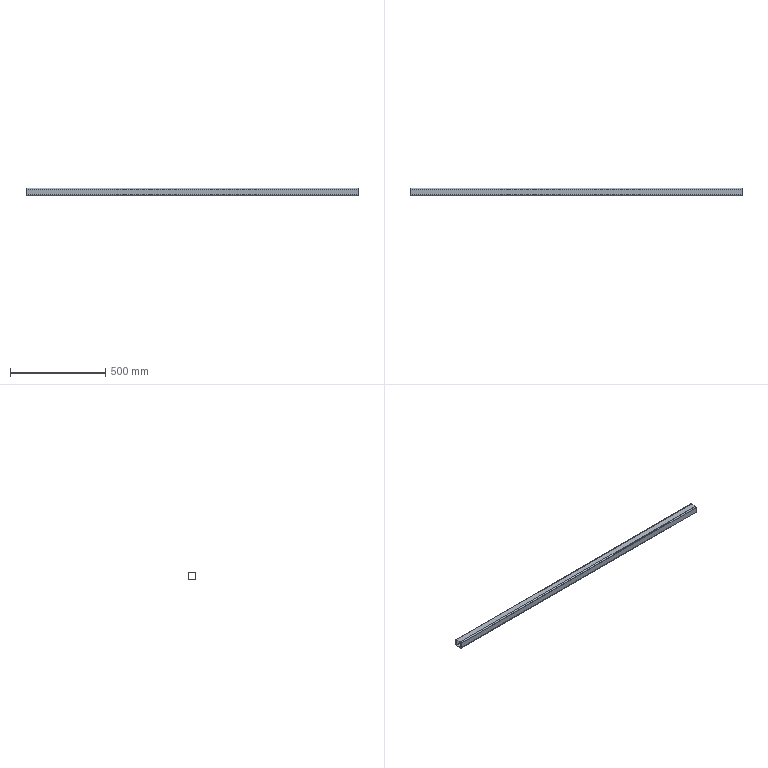Part | STEP file | SN10_002_008-04_TUBO_QUADRADO | 1 solid | 18 faces | box 1740 x 40 x 40 mm | volume 732232 mm3 | plane 10 | cylinder 8 | commonest cylinder face diameters 6 x4 12 x4
STEP:
#1=CARTESIAN_POINT('',(0.,0.,0.));
#2=DIRECTION('',(0.,0.,1.));
#3=DIRECTION('',(1.,0.,0.));
#4=AXIS2_PLACEMENT_3D('',#1,#2,#3);
#5=CARTESIAN_POINT('',(-870.,20.,14.));
#6=VERTEX_POINT('',#5);
#7=CARTESIAN_POINT('',(870.,20.,14.));
#8=VERTEX_POINT('',#7);
#9=CARTESIAN_POINT('',(-870.,20.,14.));
#10=DIRECTION('',(1.,0.,0.));
#11=VECTOR('',#10,1.);
#12=LINE('',#9,#11);
#13=CARTESIAN_POINT('',(0.,14.,14.));
#14=DIRECTION('',(1.,0.,0.));
#15=DIRECTION('',(0.,1.,0.));
#16=AXIS2_PLACEMENT_3D('',#13,#14,#15);
#17=CYLINDRICAL_SURFACE('',#16,6.);
#18=CARTESIAN_POINT('',(0.,-870.));
#19=DIRECTION('',(0.,1.));
#20=VECTOR('',#19,1.);
#21=LINE('',#18,#20);
#22=(GEOMETRIC_REPRESENTATION_CONTEXT(2)PARAMETRIC_REPRESENTATION_CONTEXT()REPRESENTATION_CONTEXT('',''));
#23=DEFINITIONAL_REPRESENTATION('',(#21),#22);
#24=PCURVE('',#17,#23);
#25=CARTESIAN_POINT('',(0.,20.,14.));
#26=DIRECTION('',(0.,-1.,0.));
#27=DIRECTION('',(0.,0.,-1.));
#28=AXIS2_PLACEMENT_3D('',#25,#26,#27);
#29=PLANE('',#28);
#30=CARTESIAN_POINT('',(0.,-870.));
#31=DIRECTION('',(0.,1.));
#32=VECTOR('',#31,1.);
#33=LINE('',#30,#32);
#34=(GEOMETRIC_REPRESENTATION_CONTEXT(2)PARAMETRIC_REPRESENTATION_CONTEXT()REPRESENTATION_CONTEXT('',''));
#35=DEFINITIONAL_REPRESENTATION('',(#33),#34);
#36=PCURVE('',#29,#35);
#37=SURFACE_CURVE('',#12,(#24,#36),.PCURVE_S1.);
#38=EDGE_CURVE('',#6,#8,#37,.T.);
#39=ORIENTED_EDGE('',*,*,#38,.F.);
#40=CARTESIAN_POINT('',(-870.,14.,20.));
#41=VERTEX_POINT('',#40);
#42=CARTESIAN_POINT('',(-870.,14.,14.));
#43=DIRECTION('',(1.,0.,0.));
#44=DIRECTION('',(0.,1.,0.));
#45=AXIS2_PLACEMENT_3D('',#42,#43,#44);
#46=CIRCLE('',#45,6.);
#47=CARTESIAN_POINT('',(0.,-870.));
#48=DIRECTION('',(1.,0.));
#49=VECTOR('',#48,1.);
#50=LINE('',#47,#49);
#51=(GEOMETRIC_REPRESENTATION_CONTEXT(2)PARAMETRIC_REPRESENTATION_CONTEXT()REPRESENTATION_CONTEXT('',''));
#52=DEFINITIONAL_REPRESENTATION('',(#50),#51);
#53=PCURVE('',#17,#52);
#54=CARTESIAN_POINT('',(-870.,0.,0.));
#55=DIRECTION('',(1.,0.,0.));
#56=DIRECTION('',(0.,0.,-1.));
#57=AXIS2_PLACEMENT_3D('',#54,#55,#56);
#58=PLANE('',#57);
#59=CARTESIAN_POINT('',(-14.,14.));
#60=DIRECTION('',(0.,1.));
#61=AXIS2_PLACEMENT_2D('',#59,#60);
#62=CIRCLE('',#61,6.);
#63=(GEOMETRIC_REPRESENTATION_CONTEXT(2)PARAMETRIC_REPRESENTATION_CONTEXT()REPRESENTATION_CONTEXT('',''));
#64=DEFINITIONAL_REPRESENTATION('',(#62),#63);
#65=PCURVE('',#58,#64);
#66=SURFACE_CURVE('',#46,(#53,#65),.PCURVE_S1.);
#67=EDGE_CURVE('',#6,#41,#66,.T.);
#68=ORIENTED_EDGE('',*,*,#67,.T.);
#69=CARTESIAN_POINT('',(870.,14.,20.));
#70=VERTEX_POINT('',#69);
#71=CARTESIAN_POINT('',(-870.,14.,20.));
#72=DIRECTION('',(1.,0.,0.));
#73=VECTOR('',#72,1.);
#74=LINE('',#71,#73);
#75=CARTESIAN_POINT('',(1.571,-870.));
#76=DIRECTION('',(0.,1.));
#77=VECTOR('',#76,1.);
#78=LINE('',#75,#77);
#79=(GEOMETRIC_REPRESENTATION_CONTEXT(2)PARAMETRIC_REPRESENTATION_CONTEXT()REPRESENTATION_CONTEXT('',''));
#80=DEFINITIONAL_REPRESENTATION('',(#78),#79);
#81=PCURVE('',#17,#80);
#82=CARTESIAN_POINT('',(0.,-14.,20.));
#83=DIRECTION('',(0.,0.,-1.));
#84=DIRECTION('',(-1.,0.,0.));
#85=AXIS2_PLACEMENT_3D('',#82,#83,#84);
#86=PLANE('',#85);
#87=CARTESIAN_POINT('',(870.,28.));
#88=DIRECTION('',(-1.,0.));
#89=VECTOR('',#88,1.);
#90=LINE('',#87,#89);
#91=(GEOMETRIC_REPRESENTATION_CONTEXT(2)PARAMETRIC_REPRESENTATION_CONTEXT()REPRESENTATION_CONTEXT('',''));
#92=DEFINITIONAL_REPRESENTATION('',(#90),#91);
#93=PCURVE('',#86,#92);
#94=SURFACE_CURVE('',#74,(#81,#93),.PCURVE_S1.);
#95=EDGE_CURVE('',#41,#70,#94,.T.);
#96=ORIENTED_EDGE('',*,*,#95,.T.);
#97=CARTESIAN_POINT('',(870.,14.,14.));
#98=DIRECTION('',(1.,0.,0.));
#99=DIRECTION('',(0.,1.,0.));
#100=AXIS2_PLACEMENT_3D('',#97,#98,#99);
#101=CIRCLE('',#100,6.);
#102=CARTESIAN_POINT('',(0.,870.));
#103=DIRECTION('',(1.,0.));
#104=VECTOR('',#103,1.);
#105=LINE('',#102,#104);
#106=(GEOMETRIC_REPRESENTATION_CONTEXT(2)PARAMETRIC_REPRESENTATION_CONTEXT()REPRESENTATION_CONTEXT('',''));
#107=DEFINITIONAL_REPRESENTATION('',(#105),#106);
#108=PCURVE('',#17,#107);
#109=CARTESIAN_POINT('',(870.,0.,0.));
#110=DIRECTION('',(1.,0.,0.));
#111=DIRECTION('',(0.,0.,-1.));
#112=AXIS2_PLACEMENT_3D('',#109,#110,#111);
#113=PLANE('',#112);
#114=CARTESIAN_POINT('',(-14.,14.));
#115=DIRECTION('',(0.,1.));
#116=AXIS2_PLACEMENT_2D('',#114,#115);
#117=CIRCLE('',#116,6.);
#118=(GEOMETRIC_REPRESENTATION_CONTEXT(2)PARAMETRIC_REPRESENTATION_CONTEXT()REPRESENTATION_CONTEXT('',''));
#119=DEFINITIONAL_REPRESENTATION('',(#117),#118);
#120=PCURVE('',#113,#119);
#121=SURFACE_CURVE('',#101,(#108,#120),.PCURVE_S1.);
#122=EDGE_CURVE('',#8,#70,#121,.T.);
#123=ORIENTED_EDGE('',*,*,#122,.F.);
#124=EDGE_LOOP('',(#39,#68,#96,#123));
#125=FACE_BOUND('',#124,.T.);
#126=ADVANCED_FACE('',(#125),#17,.T.);
#127=ORIENTED_EDGE('',*,*,#95,.F.);
#128=CARTESIAN_POINT('',(-870.,-14.,20.));
#129=VERTEX_POINT('',#128);
#130=CARTESIAN_POINT('',(-870.,-14.,20.));
#131=DIRECTION('',(0.,1.,0.));
#132=VECTOR('',#131,1.);
#133=LINE('',#130,#132);
#134=CARTESIAN_POINT('',(870.,0.));
#135=DIRECTION('',(0.,1.));
#136=VECTOR('',#135,1.);
#137=LINE('',#134,#136);
#138=(GEOMETRIC_REPRESENTATION_CONTEXT(2)PARAMETRIC_REPRESENTATION_CONTEXT()REPRESENTATION_CONTEXT('',''));
#139=DEFINITIONAL_REPRESENTATION('',(#137),#138);
#140=PCURVE('',#86,#139);
#141=CARTESIAN_POINT('',(-20.,-14.));
#142=DIRECTION('',(0.,1.));
#143=VECTOR('',#142,1.);
#144=LINE('',#141,#143);
#145=(GEOMETRIC_REPRESENTATION_CONTEXT(2)PARAMETRIC_REPRESENTATION_CONTEXT()REPRESENTATION_CONTEXT('',''));
#146=DEFINITIONAL_REPRESENTATION('',(#144),#145);
#147=PCURVE('',#58,#146);
#148=SURFACE_CURVE('',#133,(#140,#147),.PCURVE_S1.);
#149=EDGE_CURVE('',#129,#41,#148,.T.);
#150=ORIENTED_EDGE('',*,*,#149,.F.);
#151=CARTESIAN_POINT('',(870.,-14.,20.));
#152=VERTEX_POINT('',#151);
#153=CARTESIAN_POINT('',(-870.,-14.,20.));
#154=DIRECTION('',(1.,0.,0.));
#155=VECTOR('',#154,1.);
#156=LINE('',#153,#155);
#157=CARTESIAN_POINT('',(870.,0.));
#158=DIRECTION('',(-1.,0.));
#159=VECTOR('',#158,1.);
#160=LINE('',#157,#159);
#161=(GEOMETRIC_REPRESENTATION_CONTEXT(2)PARAMETRIC_REPRESENTATION_CONTEXT()REPRESENTATION_CONTEXT('',''));
#162=DEFINITIONAL_REPRESENTATION('',(#160),#161);
#163=PCURVE('',#86,#162);
#164=CARTESIAN_POINT('',(0.,-14.,14.));
#165=DIRECTION('',(1.,0.,0.));
#166=DIRECTION('',(0.,0.,1.));
#167=AXIS2_PLACEMENT_3D('',#164,#165,#166);
#168=CYLINDRICAL_SURFACE('',#167,6.);
#169=CARTESIAN_POINT('',(0.,-870.));
#170=DIRECTION('',(0.,1.));
#171=VECTOR('',#170,1.);
#172=LINE('',#169,#171);
#173=(GEOMETRIC_REPRESENTATION_CONTEXT(2)PARAMETRIC_REPRESENTATION_CONTEXT()REPRESENTATION_CONTEXT('',''));
#174=DEFINITIONAL_REPRESENTATION('',(#172),#173);
#175=PCURVE('',#168,#174);
#176=SURFACE_CURVE('',#156,(#163,#175),.PCURVE_S1.);
#177=EDGE_CURVE('',#129,#152,#176,.T.);
#178=ORIENTED_EDGE('',*,*,#177,.T.);
#179=CARTESIAN_POINT('',(870.,-14.,20.));
#180=DIRECTION('',(0.,1.,0.));
#181=VECTOR('',#180,1.);
#182=LINE('',#179,#181);
#183=CARTESIAN_POINT('',(-870.,0.));
#184=DIRECTION('',(0.,1.));
#185=VECTOR('',#184,1.);
#186=LINE('',#183,#185);
#187=(GEOMETRIC_REPRESENTATION_CONTEXT(2)PARAMETRIC_REPRESENTATION_CONTEXT()REPRESENTATION_CONTEXT('',''));
#188=DEFINITIONAL_REPRESENTATION('',(#186),#187);
#189=PCURVE('',#86,#188);
#190=CARTESIAN_POINT('',(-20.,-14.));
#191=DIRECTION('',(0.,1.));
#192=VECTOR('',#191,1.);
#193=LINE('',#190,#192);
#194=(GEOMETRIC_REPRESENTATION_CONTEXT(2)PARAMETRIC_REPRESENTATION_CONTEXT()REPRESENTATION_CONTEXT('',''));
#195=DEFINITIONAL_REPRESENTATION('',(#193),#194);
#196=PCURVE('',#113,#195);
#197=SURFACE_CURVE('',#182,(#189,#196),.PCURVE_S1.);
#198=EDGE_CURVE('',#152,#70,#197,.T.);
#199=ORIENTED_EDGE('',*,*,#198,.T.);
#200=EDGE_LOOP('',(#127,#150,#178,#199));
#201=FACE_BOUND('',#200,.T.);
#202=ADVANCED_FACE('',(#201),#86,.F.);
#203=ORIENTED_EDGE('',*,*,#177,.F.);
#204=CARTESIAN_POINT('',(-870.,-20.,14.));
#205=VERTEX_POINT('',#204);
#206=CARTESIAN_POINT('',(-870.,-14.,14.));
#207=DIRECTION('',(1.,0.,0.));
#208=DIRECTION('',(0.,1.,0.));
#209=AXIS2_PLACEMENT_3D('',#206,#207,#208);
#210=CIRCLE('',#209,6.);
#211=CARTESIAN_POINT('',(-1.571,-870.));
#212=DIRECTION('',(1.,0.));
#213=VECTOR('',#212,1.);
#214=LINE('',#211,#213);
#215=(GEOMETRIC_REPRESENTATION_CONTEXT(2)PARAMETRIC_REPRESENTATION_CONTEXT()REPRESENTATION_CONTEXT('',''));
#216=DEFINITIONAL_REPRESENTATION('',(#214),#215);
#217=PCURVE('',#168,#216);
#218=CARTESIAN_POINT('',(-14.,-14.));
#219=DIRECTION('',(0.,1.));
#220=AXIS2_PLACEMENT_2D('',#218,#219);
#221=CIRCLE('',#220,6.);
#222=(GEOMETRIC_REPRESENTATION_CONTEXT(2)PARAMETRIC_REPRESENTATION_CONTEXT()REPRESENTATION_CONTEXT('',''));
#223=DEFINITIONAL_REPRESENTATION('',(#221),#222);
#224=PCURVE('',#58,#223);
#225=SURFACE_CURVE('',#210,(#217,#224),.PCURVE_S1.);
#226=EDGE_CURVE('',#129,#205,#225,.T.);
#227=ORIENTED_EDGE('',*,*,#226,.T.);
#228=CARTESIAN_POINT('',(870.,-20.,14.));
#229=VERTEX_POINT('',#228);
#230=CARTESIAN_POINT('',(-870.,-20.,14.));
#231=DIRECTION('',(1.,0.,0.));
#232=VECTOR('',#231,1.);
#233=LINE('',#230,#232);
#234=CARTESIAN_POINT('',(1.571,-870.));
#235=DIRECTION('',(0.,1.));
#236=VECTOR('',#235,1.);
#237=LINE('',#234,#236);
#238=(GEOMETRIC_REPRESENTATION_CONTEXT(2)PARAMETRIC_REPRESENTATION_CONTEXT()REPRESENTATION_CONTEXT('',''));
#239=DEFINITIONAL_REPRESENTATION('',(#237),#238);
#240=PCURVE('',#168,#239);
#241=CARTESIAN_POINT('',(0.,-20.,-14.));
#242=DIRECTION('',(0.,1.,0.));
#243=DIRECTION('',(0.,0.,1.));
#244=AXIS2_PLACEMENT_3D('',#241,#242,#243);
#245=PLANE('',#244);
#246=CARTESIAN_POINT('',(28.,-870.));
#247=DIRECTION('',(0.,1.));
#248=VECTOR('',#247,1.);
#249=LINE('',#246,#248);
#250=(GEOMETRIC_REPRESENTATION_CONTEXT(2)PARAMETRIC_REPRESENTATION_CONTEXT()REPRESENTATION_CONTEXT('',''));
#251=DEFINITIONAL_REPRESENTATION('',(#249),#250);
#252=PCURVE('',#245,#251);
#253=SURFACE_CURVE('',#233,(#240,#252),.PCURVE_S1.);
#254=EDGE_CURVE('',#205,#229,#253,.T.);
#255=ORIENTED_EDGE('',*,*,#254,.T.);
#256=CARTESIAN_POINT('',(870.,-14.,14.));
#257=DIRECTION('',(1.,0.,0.));
#258=DIRECTION('',(0.,1.,0.));
#259=AXIS2_PLACEMENT_3D('',#256,#257,#258);
#260=CIRCLE('',#259,6.);
#261=CARTESIAN_POINT('',(-1.571,870.));
#262=DIRECTION('',(1.,0.));
#263=VECTOR('',#262,1.);
#264=LINE('',#261,#263);
#265=(GEOMETRIC_REPRESENTATION_CONTEXT(2)PARAMETRIC_REPRESENTATION_CONTEXT()REPRESENTATION_CONTEXT('',''));
#266=DEFINITIONAL_REPRESENTATION('',(#264),#265);
#267=PCURVE('',#168,#266);
#268=CARTESIAN_POINT('',(-14.,-14.));
#269=DIRECTION('',(0.,1.));
#270=AXIS2_PLACEMENT_2D('',#268,#269);
#271=CIRCLE('',#270,6.);
#272=(GEOMETRIC_REPRESENTATION_CONTEXT(2)PARAMETRIC_REPRESENTATION_CONTEXT()REPRESENTATION_CONTEXT('',''));
#273=DEFINITIONAL_REPRESENTATION('',(#271),#272);
#274=PCURVE('',#113,#273);
#275=SURFACE_CURVE('',#260,(#267,#274),.PCURVE_S1.);
#276=EDGE_CURVE('',#152,#229,#275,.T.);
#277=ORIENTED_EDGE('',*,*,#276,.F.);
#278=EDGE_LOOP('',(#203,#227,#255,#277));
#279=FACE_BOUND('',#278,.T.);
#280=ADVANCED_FACE('',(#279),#168,.T.);
#281=ORIENTED_EDGE('',*,*,#254,.F.);
#282=CARTESIAN_POINT('',(-870.,-20.,-14.));
#283=VERTEX_POINT('',#282);
#284=CARTESIAN_POINT('',(-870.,-20.,-14.));
#285=DIRECTION('',(0.,0.,1.));
#286=VECTOR('',#285,1.);
#287=LINE('',#284,#286);
#288=CARTESIAN_POINT('',(0.,-870.));
#289=DIRECTION('',(1.,0.));
#290=VECTOR('',#289,1.);
#291=LINE('',#288,#290);
#292=(GEOMETRIC_REPRESENTATION_CONTEXT(2)PARAMETRIC_REPRESENTATION_CONTEXT()REPRESENTATION_CONTEXT('',''));
#293=DEFINITIONAL_REPRESENTATION('',(#291),#292);
#294=PCURVE('',#245,#293);
#295=CARTESIAN_POINT('',(14.,-20.));
#296=DIRECTION('',(-1.,0.));
#297=VECTOR('',#296,1.);
#298=LINE('',#295,#297);
#299=(GEOMETRIC_REPRESENTATION_CONTEXT(2)PARAMETRIC_REPRESENTATION_CONTEXT()REPRESENTATION_CONTEXT('',''));
#300=DEFINITIONAL_REPRESENTATION('',(#298),#299);
#301=PCURVE('',#58,#300);
#302=SURFACE_CURVE('',#287,(#294,#301),.PCURVE_S1.);
#303=EDGE_CURVE('',#283,#205,#302,.T.);
#304=ORIENTED_EDGE('',*,*,#303,.F.);
#305=CARTESIAN_POINT('',(870.,-20.,-14.));
#306=VERTEX_POINT('',#305);
#307=CARTESIAN_POINT('',(-870.,-20.,-14.));
#308=DIRECTION('',(1.,0.,0.));
#309=VECTOR('',#308,1.);
#310=LINE('',#307,#309);
#311=CARTESIAN_POINT('',(0.,-870.));
#312=DIRECTION('',(0.,1.));
#313=VECTOR('',#312,1.);
#314=LINE('',#311,#313);
#315=(GEOMETRIC_REPRESENTATION_CONTEXT(2)PARAMETRIC_REPRESENTATION_CONTEXT()REPRESENTATION_CONTEXT('',''));
#316=DEFINITIONAL_REPRESENTATION('',(#314),#315);
#317=PCURVE('',#245,#316);
#318=CARTESIAN_POINT('',(0.,-14.,-14.));
#319=DIRECTION('',(1.,0.,0.));
#320=DIRECTION('',(0.,-1.,0.));
#321=AXIS2_PLACEMENT_3D('',#318,#319,#320);
#322=CYLINDRICAL_SURFACE('',#321,6.);
#323=CARTESIAN_POINT('',(0.,-870.));
#324=DIRECTION('',(0.,1.));
#325=VECTOR('',#324,1.);
#326=LINE('',#323,#325);
#327=(GEOMETRIC_REPRESENTATION_CONTEXT(2)PARAMETRIC_REPRESENTATION_CONTEXT()REPRESENTATION_CONTEXT('',''));
#328=DEFINITIONAL_REPRESENTATION('',(#326),#327);
#329=PCURVE('',#322,#328);
#330=SURFACE_CURVE('',#310,(#317,#329),.PCURVE_S1.);
#331=EDGE_CURVE('',#283,#306,#330,.T.);
#332=ORIENTED_EDGE('',*,*,#331,.T.);
#333=CARTESIAN_POINT('',(870.,-20.,-14.));
#334=DIRECTION('',(0.,0.,1.));
#335=VECTOR('',#334,1.);
#336=LINE('',#333,#335);
#337=CARTESIAN_POINT('',(0.,870.));
#338=DIRECTION('',(1.,0.));
#339=VECTOR('',#338,1.);
#340=LINE('',#337,#339);
#341=(GEOMETRIC_REPRESENTATION_CONTEXT(2)PARAMETRIC_REPRESENTATION_CONTEXT()REPRESENTATION_CONTEXT('',''));
#342=DEFINITIONAL_REPRESENTATION('',(#340),#341);
#343=PCURVE('',#245,#342);
#344=CARTESIAN_POINT('',(14.,-20.));
#345=DIRECTION('',(-1.,0.));
#346=VECTOR('',#345,1.);
#347=LINE('',#344,#346);
#348=(GEOMETRIC_REPRESENTATION_CONTEXT(2)PARAMETRIC_REPRESENTATION_CONTEXT()REPRESENTATION_CONTEXT('',''));
#349=DEFINITIONAL_REPRESENTATION('',(#347),#348);
#350=PCURVE('',#113,#349);
#351=SURFACE_CURVE('',#336,(#343,#350),.PCURVE_S1.);
#352=EDGE_CURVE('',#306,#229,#351,.T.);
#353=ORIENTED_EDGE('',*,*,#352,.T.);
#354=EDGE_LOOP('',(#281,#304,#332,#353));
#355=FACE_BOUND('',#354,.T.);
#356=ADVANCED_FACE('',(#355),#245,.F.);
#357=ORIENTED_EDGE('',*,*,#331,.F.);
#358=CARTESIAN_POINT('',(-870.,-14.,-20.));
#359=VERTEX_POINT('',#358);
#360=CARTESIAN_POINT('',(-870.,-14.,-14.));
#361=DIRECTION('',(1.,0.,0.));
#362=DIRECTION('',(0.,1.,0.));
#363=AXIS2_PLACEMENT_3D('',#360,#361,#362);
#364=CIRCLE('',#363,6.);
#365=CARTESIAN_POINT('',(-3.142,-870.));
#366=DIRECTION('',(1.,0.));
#367=VECTOR('',#366,1.);
#368=LINE('',#365,#367);
#369=(GEOMETRIC_REPRESENTATION_CONTEXT(2)PARAMETRIC_REPRESENTATION_CONTEXT()REPRESENTATION_CONTEXT('',''));
#370=DEFINITIONAL_REPRESENTATION('',(#368),#369);
#371=PCURVE('',#322,#370);
#372=CARTESIAN_POINT('',(14.,-14.));
#373=DIRECTION('',(0.,1.));
#374=AXIS2_PLACEMENT_2D('',#372,#373);
#375=CIRCLE('',#374,6.);
#376=(GEOMETRIC_REPRESENTATION_CONTEXT(2)PARAMETRIC_REPRESENTATION_CONTEXT()REPRESENTATION_CONTEXT('',''));
#377=DEFINITIONAL_REPRESENTATION('',(#375),#376);
#378=PCURVE('',#58,#377);
#379=SURFACE_CURVE('',#364,(#371,#378),.PCURVE_S1.);
#380=EDGE_CURVE('',#283,#359,#379,.T.);
#381=ORIENTED_EDGE('',*,*,#380,.T.);
#382=CARTESIAN_POINT('',(870.,-14.,-20.));
#383=VERTEX_POINT('',#382);
#384=CARTESIAN_POINT('',(-870.,-14.,-20.));
#385=DIRECTION('',(1.,0.,0.));
#386=VECTOR('',#385,1.);
#387=LINE('',#384,#386);
#388=CARTESIAN_POINT('',(1.571,-870.));
#389=DIRECTION('',(0.,1.));
#390=VECTOR('',#389,1.);
#391=LINE('',#388,#390);
#392=(GEOMETRIC_REPRESENTATION_CONTEXT(2)PARAMETRIC_REPRESENTATION_CONTEXT()REPRESENTATION_CONTEXT('',''));
#393=DEFINITIONAL_REPRESENTATION('',(#391),#392);
#394=PCURVE('',#322,#393);
#395=CARTESIAN_POINT('',(0.,14.,-20.));
#396=DIRECTION('',(0.,0.,1.));
#397=DIRECTION('',(1.,0.,0.));
#398=AXIS2_PLACEMENT_3D('',#395,#396,#397);
#399=PLANE('',#398);
#400=CARTESIAN_POINT('',(-870.,-28.));
#401=DIRECTION('',(1.,0.));
#402=VECTOR('',#401,1.);
#403=LINE('',#400,#402);
#404=(GEOMETRIC_REPRESENTATION_CONTEXT(2)PARAMETRIC_REPRESENTATION_CONTEXT()REPRESENTATION_CONTEXT('',''));
#405=DEFINITIONAL_REPRESENTATION('',(#403),#404);
#406=PCURVE('',#399,#405);
#407=SURFACE_CURVE('',#387,(#394,#406),.PCURVE_S1.);
#408=EDGE_CURVE('',#359,#383,#407,.T.);
#409=ORIENTED_EDGE('',*,*,#408,.T.);
#410=CARTESIAN_POINT('',(870.,-14.,-14.));
#411=DIRECTION('',(1.,0.,0.));
#412=DIRECTION('',(0.,1.,0.));
#413=AXIS2_PLACEMENT_3D('',#410,#411,#412);
#414=CIRCLE('',#413,6.);
#415=CARTESIAN_POINT('',(-3.142,870.));
#416=DIRECTION('',(1.,0.));
#417=VECTOR('',#416,1.);
#418=LINE('',#415,#417);
#419=(GEOMETRIC_REPRESENTATION_CONTEXT(2)PARAMETRIC_REPRESENTATION_CONTEXT()REPRESENTATION_CONTEXT('',''));
#420=DEFINITIONAL_REPRESENTATION('',(#418),#419);
#421=PCURVE('',#322,#420);
#422=CARTESIAN_POINT('',(14.,-14.));
#423=DIRECTION('',(0.,1.));
#424=AXIS2_PLACEMENT_2D('',#422,#423);
#425=CIRCLE('',#424,6.);
#426=(GEOMETRIC_REPRESENTATION_CONTEXT(2)PARAMETRIC_REPRESENTATION_CONTEXT()REPRESENTATION_CONTEXT('',''));
#427=DEFINITIONAL_REPRESENTATION('',(#425),#426);
#428=PCURVE('',#113,#427);
#429=SURFACE_CURVE('',#414,(#421,#428),.PCURVE_S1.);
#430=EDGE_CURVE('',#306,#383,#429,.T.);
#431=ORIENTED_EDGE('',*,*,#430,.F.);
#432=EDGE_LOOP('',(#357,#381,#409,#431));
#433=FACE_BOUND('',#432,.T.);
#434=ADVANCED_FACE('',(#433),#322,.T.);
#435=ORIENTED_EDGE('',*,*,#408,.F.);
#436=CARTESIAN_POINT('',(-870.,14.,-20.));
#437=VERTEX_POINT('',#436);
#438=CARTESIAN_POINT('',(-870.,14.,-20.));
#439=DIRECTION('',(0.,-1.,0.));
#440=VECTOR('',#439,1.);
#441=LINE('',#438,#440);
#442=CARTESIAN_POINT('',(-870.,0.));
#443=DIRECTION('',(0.,-1.));
#444=VECTOR('',#443,1.);
#445=LINE('',#442,#444);
#446=(GEOMETRIC_REPRESENTATION_CONTEXT(2)PARAMETRIC_REPRESENTATION_CONTEXT()REPRESENTATION_CONTEXT('',''));
#447=DEFINITIONAL_REPRESENTATION('',(#445),#446);
#448=PCURVE('',#399,#447);
#449=CARTESIAN_POINT('',(20.,14.));
#450=DIRECTION('',(0.,-1.));
#451=VECTOR('',#450,1.);
#452=LINE('',#449,#451);
#453=(GEOMETRIC_REPRESENTATION_CONTEXT(2)PARAMETRIC_REPRESENTATION_CONTEXT()REPRESENTATION_CONTEXT('',''));
#454=DEFINITIONAL_REPRESENTATION('',(#452),#453);
#455=PCURVE('',#58,#454);
#456=SURFACE_CURVE('',#441,(#448,#455),.PCURVE_S1.);
#457=EDGE_CURVE('',#437,#359,#456,.T.);
#458=ORIENTED_EDGE('',*,*,#457,.F.);
#459=CARTESIAN_POINT('',(870.,14.,-20.));
#460=VERTEX_POINT('',#459);
#461=CARTESIAN_POINT('',(-870.,14.,-20.));
#462=DIRECTION('',(1.,0.,0.));
#463=VECTOR('',#462,1.);
#464=LINE('',#461,#463);
#465=CARTESIAN_POINT('',(-870.,0.));
#466=DIRECTION('',(1.,0.));
#467=VECTOR('',#466,1.);
#468=LINE('',#465,#467);
#469=(GEOMETRIC_REPRESENTATION_CONTEXT(2)PARAMETRIC_REPRESENTATION_CONTEXT()REPRESENTATION_CONTEXT('',''));
#470=DEFINITIONAL_REPRESENTATION('',(#468),#469);
#471=PCURVE('',#399,#470);
#472=CARTESIAN_POINT('',(0.,14.,-14.));
#473=DIRECTION('',(1.,0.,0.));
#474=DIRECTION('',(0.,0.,-1.));
#475=AXIS2_PLACEMENT_3D('',#472,#473,#474);
#476=CYLINDRICAL_SURFACE('',#475,6.);
#477=CARTESIAN_POINT('',(0.,-870.));
#478=DIRECTION('',(0.,1.));
#479=VECTOR('',#478,1.);
#480=LINE('',#477,#479);
#481=(GEOMETRIC_REPRESENTATION_CONTEXT(2)PARAMETRIC_REPRESENTATION_CONTEXT()REPRESENTATION_CONTEXT('',''));
#482=DEFINITIONAL_REPRESENTATION('',(#480),#481);
#483=PCURVE('',#476,#482);
#484=SURFACE_CURVE('',#464,(#471,#483),.PCURVE_S1.);
#485=EDGE_CURVE('',#437,#460,#484,.T.);
#486=ORIENTED_EDGE('',*,*,#485,.T.);
#487=CARTESIAN_POINT('',(870.,14.,-20.));
#488=DIRECTION('',(0.,-1.,0.));
#489=VECTOR('',#488,1.);
#490=LINE('',#487,#489);
#491=CARTESIAN_POINT('',(870.,0.));
#492=DIRECTION('',(0.,-1.));
#493=VECTOR('',#492,1.);
#494=LINE('',#491,#493);
#495=(GEOMETRIC_REPRESENTATION_CONTEXT(2)PARAMETRIC_REPRESENTATION_CONTEXT()REPRESENTATION_CONTEXT('',''));
#496=DEFINITIONAL_REPRESENTATION('',(#494),#495);
#497=PCURVE('',#399,#496);
#498=CARTESIAN_POINT('',(20.,14.));
#499=DIRECTION('',(0.,-1.));
#500=VECTOR('',#499,1.);
#501=LINE('',#498,#500);
#502=(GEOMETRIC_REPRESENTATION_CONTEXT(2)PARAMETRIC_REPRESENTATION_CONTEXT()REPRESENTATION_CONTEXT('',''));
#503=DEFINITIONAL_REPRESENTATION('',(#501),#502);
#504=PCURVE('',#113,#503);
#505=SURFACE_CURVE('',#490,(#497,#504),.PCURVE_S1.);
#506=EDGE_CURVE('',#460,#383,#505,.T.);
#507=ORIENTED_EDGE('',*,*,#506,.T.);
#508=EDGE_LOOP('',(#435,#458,#486,#507));
#509=FACE_BOUND('',#508,.T.);
#510=ADVANCED_FACE('',(#509),#399,.F.);
#511=ORIENTED_EDGE('',*,*,#485,.F.);
#512=CARTESIAN_POINT('',(-870.,20.,-14.));
#513=VERTEX_POINT('',#512);
#514=CARTESIAN_POINT('',(-870.,14.,-14.));
#515=DIRECTION('',(1.,0.,0.));
#516=DIRECTION('',(0.,1.,0.));
#517=AXIS2_PLACEMENT_3D('',#514,#515,#516);
#518=CIRCLE('',#517,6.);
#519=CARTESIAN_POINT('',(-4.712,-870.));
#520=DIRECTION('',(1.,0.));
#521=VECTOR('',#520,1.);
#522=LINE('',#519,#521);
#523=(GEOMETRIC_REPRESENTATION_CONTEXT(2)PARAMETRIC_REPRESENTATION_CONTEXT()REPRESENTATION_CONTEXT('',''));
#524=DEFINITIONAL_REPRESENTATION('',(#522),#523);
#525=PCURVE('',#476,#524);
#526=CARTESIAN_POINT('',(14.,14.));
#527=DIRECTION('',(0.,1.));
#528=AXIS2_PLACEMENT_2D('',#526,#527);
#529=CIRCLE('',#528,6.);
#530=(GEOMETRIC_REPRESENTATION_CONTEXT(2)PARAMETRIC_REPRESENTATION_CONTEXT()REPRESENTATION_CONTEXT('',''));
#531=DEFINITIONAL_REPRESENTATION('',(#529),#530);
#532=PCURVE('',#58,#531);
#533=SURFACE_CURVE('',#518,(#525,#532),.PCURVE_S1.);
#534=EDGE_CURVE('',#437,#513,#533,.T.);
#535=ORIENTED_EDGE('',*,*,#534,.T.);
#536=CARTESIAN_POINT('',(870.,20.,-14.));
#537=VERTEX_POINT('',#536);
#538=CARTESIAN_POINT('',(-870.,20.,-14.));
#539=DIRECTION('',(1.,0.,0.));
#540=VECTOR('',#539,1.);
#541=LINE('',#538,#540);
#542=CARTESIAN_POINT('',(1.571,-870.));
#543=DIRECTION('',(0.,1.));
#544=VECTOR('',#543,1.);
#545=LINE('',#542,#544);
#546=(GEOMETRIC_REPRESENTATION_CONTEXT(2)PARAMETRIC_REPRESENTATION_CONTEXT()REPRESENTATION_CONTEXT('',''));
#547=DEFINITIONAL_REPRESENTATION('',(#545),#546);
#548=PCURVE('',#476,#547);
#549=CARTESIAN_POINT('',(28.,-870.));
#550=DIRECTION('',(0.,1.));
#551=VECTOR('',#550,1.);
#552=LINE('',#549,#551);
#553=(GEOMETRIC_REPRESENTATION_CONTEXT(2)PARAMETRIC_REPRESENTATION_CONTEXT()REPRESENTATION_CONTEXT('',''));
#554=DEFINITIONAL_REPRESENTATION('',(#552),#553);
#555=PCURVE('',#29,#554);
#556=SURFACE_CURVE('',#541,(#548,#555),.PCURVE_S1.);
#557=EDGE_CURVE('',#513,#537,#556,.T.);
#558=ORIENTED_EDGE('',*,*,#557,.T.);
#559=CARTESIAN_POINT('',(870.,14.,-14.));
#560=DIRECTION('',(1.,0.,0.));
#561=DIRECTION('',(0.,1.,0.));
#562=AXIS2_PLACEMENT_3D('',#559,#560,#561);
#563=CIRCLE('',#562,6.);
#564=CARTESIAN_POINT('',(-4.712,870.));
#565=DIRECTION('',(1.,0.));
#566=VECTOR('',#565,1.);
#567=LINE('',#564,#566);
#568=(GEOMETRIC_REPRESENTATION_CONTEXT(2)PARAMETRIC_REPRESENTATION_CONTEXT()REPRESENTATION_CONTEXT('',''));
#569=DEFINITIONAL_REPRESENTATION('',(#567),#568);
#570=PCURVE('',#476,#569);
#571=CARTESIAN_POINT('',(14.,14.));
#572=DIRECTION('',(0.,1.));
#573=AXIS2_PLACEMENT_2D('',#571,#572);
#574=CIRCLE('',#573,6.);
#575=(GEOMETRIC_REPRESENTATION_CONTEXT(2)PARAMETRIC_REPRESENTATION_CONTEXT()REPRESENTATION_CONTEXT('',''));
#576=DEFINITIONAL_REPRESENTATION('',(#574),#575);
#577=PCURVE('',#113,#576);
#578=SURFACE_CURVE('',#563,(#570,#577),.PCURVE_S1.);
#579=EDGE_CURVE('',#460,#537,#578,.T.);
#580=ORIENTED_EDGE('',*,*,#579,.F.);
#581=EDGE_LOOP('',(#511,#535,#558,#580));
#582=FACE_BOUND('',#581,.T.);
#583=ADVANCED_FACE('',(#582),#476,.T.);
#584=ORIENTED_EDGE('',*,*,#557,.F.);
#585=CARTESIAN_POINT('',(-870.,20.,14.));
#586=DIRECTION('',(0.,0.,-1.));
#587=VECTOR('',#586,1.);
#588=LINE('',#585,#587);
#589=CARTESIAN_POINT('',(0.,-870.));
#590=DIRECTION('',(1.,0.));
#591=VECTOR('',#590,1.);
#592=LINE('',#589,#591);
#593=(GEOMETRIC_REPRESENTATION_CONTEXT(2)PARAMETRIC_REPRESENTATION_CONTEXT()REPRESENTATION_CONTEXT('',''));
#594=DEFINITIONAL_REPRESENTATION('',(#592),#593);
#595=PCURVE('',#29,#594);
#596=CARTESIAN_POINT('',(-14.,20.));
#597=DIRECTION('',(1.,0.));
#598=VECTOR('',#597,1.);
#599=LINE('',#596,#598);
#600=(GEOMETRIC_REPRESENTATION_CONTEXT(2)PARAMETRIC_REPRESENTATION_CONTEXT()REPRESENTATION_CONTEXT('',''));
#601=DEFINITIONAL_REPRESENTATION('',(#599),#600);
#602=PCURVE('',#58,#601);
#603=SURFACE_CURVE('',#588,(#595,#602),.PCURVE_S1.);
#604=EDGE_CURVE('',#6,#513,#603,.T.);
#605=ORIENTED_EDGE('',*,*,#604,.F.);
#606=ORIENTED_EDGE('',*,*,#38,.T.);
#607=CARTESIAN_POINT('',(870.,20.,14.));
#608=DIRECTION('',(0.,0.,-1.));
#609=VECTOR('',#608,1.);
#610=LINE('',#607,#609);
#611=CARTESIAN_POINT('',(0.,870.));
#612=DIRECTION('',(1.,0.));
#613=VECTOR('',#612,1.);
#614=LINE('',#611,#613);
#615=(GEOMETRIC_REPRESENTATION_CONTEXT(2)PARAMETRIC_REPRESENTATION_CONTEXT()REPRESENTATION_CONTEXT('',''));
#616=DEFINITIONAL_REPRESENTATION('',(#614),#615);
#617=PCURVE('',#29,#616);
#618=CARTESIAN_POINT('',(-14.,20.));
#619=DIRECTION('',(1.,0.));
#620=VECTOR('',#619,1.);
#621=LINE('',#618,#620);
#622=(GEOMETRIC_REPRESENTATION_CONTEXT(2)PARAMETRIC_REPRESENTATION_CONTEXT()REPRESENTATION_CONTEXT('',''));
#623=DEFINITIONAL_REPRESENTATION('',(#621),#622);
#624=PCURVE('',#113,#623);
#625=SURFACE_CURVE('',#610,(#617,#624),.PCURVE_S1.);
#626=EDGE_CURVE('',#8,#537,#625,.T.);
#627=ORIENTED_EDGE('',*,*,#626,.T.);
#628=EDGE_LOOP('',(#584,#605,#606,#627));
#629=FACE_BOUND('',#628,.T.);
#630=ADVANCED_FACE('',(#629),#29,.F.);
#631=CARTESIAN_POINT('',(870.,17.,14.));
#632=VERTEX_POINT('',#631);
#633=CARTESIAN_POINT('',(870.,17.,-14.));
#634=VERTEX_POINT('',#633);
#635=CARTESIAN_POINT('',(870.,17.,14.));
#636=DIRECTION('',(0.,0.,-1.));
#637=VECTOR('',#636,1.);
#638=LINE('',#635,#637);
#639=CARTESIAN_POINT('',(0.,17.,14.));
#640=DIRECTION('',(0.,-1.,0.));
#641=DIRECTION('',(0.,0.,-1.));
#642=AXIS2_PLACEMENT_3D('',#639,#640,#641);
#643=PLANE('',#642);
#644=CARTESIAN_POINT('',(0.,870.));
#645=DIRECTION('',(1.,0.));
#646=VECTOR('',#645,1.);
#647=LINE('',#644,#646);
#648=(GEOMETRIC_REPRESENTATION_CONTEXT(2)PARAMETRIC_REPRESENTATION_CONTEXT()REPRESENTATION_CONTEXT('',''));
#649=DEFINITIONAL_REPRESENTATION('',(#647),#648);
#650=PCURVE('',#643,#649);
#651=CARTESIAN_POINT('',(-14.,17.));
#652=DIRECTION('',(1.,0.));
#653=VECTOR('',#652,1.);
#654=LINE('',#651,#653);
#655=(GEOMETRIC_REPRESENTATION_CONTEXT(2)PARAMETRIC_REPRESENTATION_CONTEXT()REPRESENTATION_CONTEXT('',''));
#656=DEFINITIONAL_REPRESENTATION('',(#654),#655);
#657=PCURVE('',#113,#656);
#658=SURFACE_CURVE('',#638,(#650,#657),.PCURVE_S1.);
#659=EDGE_CURVE('',#632,#634,#658,.T.);
#660=ORIENTED_EDGE('',*,*,#659,.F.);
#661=CARTESIAN_POINT('',(-870.,17.,14.));
#662=VERTEX_POINT('',#661);
#663=CARTESIAN_POINT('',(-870.,17.,14.));
#664=DIRECTION('',(1.,0.,0.));
#665=VECTOR('',#664,1.);
#666=LINE('',#663,#665);
#667=CARTESIAN_POINT('',(0.,-870.));
#668=DIRECTION('',(0.,1.));
#669=VECTOR('',#668,1.);
#670=LINE('',#667,#669);
#671=(GEOMETRIC_REPRESENTATION_CONTEXT(2)PARAMETRIC_REPRESENTATION_CONTEXT()REPRESENTATION_CONTEXT('',''));
#672=DEFINITIONAL_REPRESENTATION('',(#670),#671);
#673=PCURVE('',#643,#672);
#674=CARTESIAN_POINT('',(0.,14.,14.));
#675=DIRECTION('',(1.,0.,0.));
#676=DIRECTION('',(0.,1.,0.));
#677=AXIS2_PLACEMENT_3D('',#674,#675,#676);
#678=CYLINDRICAL_SURFACE('',#677,3.);
#679=CARTESIAN_POINT('',(0.,-870.));
#680=DIRECTION('',(0.,1.));
#681=VECTOR('',#680,1.);
#682=LINE('',#679,#681);
#683=(GEOMETRIC_REPRESENTATION_CONTEXT(2)PARAMETRIC_REPRESENTATION_CONTEXT()REPRESENTATION_CONTEXT('',''));
#684=DEFINITIONAL_REPRESENTATION('',(#682),#683);
#685=PCURVE('',#678,#684);
#686=SURFACE_CURVE('',#666,(#673,#685),.PCURVE_S1.);
#687=EDGE_CURVE('',#662,#632,#686,.T.);
#688=ORIENTED_EDGE('',*,*,#687,.F.);
#689=CARTESIAN_POINT('',(-870.,17.,-14.));
#690=VERTEX_POINT('',#689);
#691=CARTESIAN_POINT('',(-870.,17.,14.));
#692=DIRECTION('',(0.,0.,-1.));
#693=VECTOR('',#692,1.);
#694=LINE('',#691,#693);
#695=CARTESIAN_POINT('',(0.,-870.));
#696=DIRECTION('',(1.,0.));
#697=VECTOR('',#696,1.);
#698=LINE('',#695,#697);
#699=(GEOMETRIC_REPRESENTATION_CONTEXT(2)PARAMETRIC_REPRESENTATION_CONTEXT()REPRESENTATION_CONTEXT('',''));
#700=DEFINITIONAL_REPRESENTATION('',(#698),#699);
#701=PCURVE('',#643,#700);
#702=CARTESIAN_POINT('',(-14.,17.));
#703=DIRECTION('',(1.,0.));
#704=VECTOR('',#703,1.);
#705=LINE('',#702,#704);
#706=(GEOMETRIC_REPRESENTATION_CONTEXT(2)PARAMETRIC_REPRESENTATION_CONTEXT()REPRESENTATION_CONTEXT('',''));
#707=DEFINITIONAL_REPRESENTATION('',(#705),#706);
#708=PCURVE('',#58,#707);
#709=SURFACE_CURVE('',#694,(#701,#708),.PCURVE_S1.);
#710=EDGE_CURVE('',#662,#690,#709,.T.);
#711=ORIENTED_EDGE('',*,*,#710,.T.);
#712=CARTESIAN_POINT('',(-870.,17.,-14.));
#713=DIRECTION('',(1.,0.,0.));
#714=VECTOR('',#713,1.);
#715=LINE('',#712,#714);
#716=CARTESIAN_POINT('',(28.,-870.));
#717=DIRECTION('',(0.,1.));
#718=VECTOR('',#717,1.);
#719=LINE('',#716,#718);
#720=(GEOMETRIC_REPRESENTATION_CONTEXT(2)PARAMETRIC_REPRESENTATION_CONTEXT()REPRESENTATION_CONTEXT('',''));
#721=DEFINITIONAL_REPRESENTATION('',(#719),#720);
#722=PCURVE('',#643,#721);
#723=CARTESIAN_POINT('',(0.,14.,-14.));
#724=DIRECTION('',(1.,0.,0.));
#725=DIRECTION('',(0.,0.,-1.));
#726=AXIS2_PLACEMENT_3D('',#723,#724,#725);
#727=CYLINDRICAL_SURFACE('',#726,3.);
#728=CARTESIAN_POINT('',(1.571,-870.));
#729=DIRECTION('',(0.,1.));
#730=VECTOR('',#729,1.);
#731=LINE('',#728,#730);
#732=(GEOMETRIC_REPRESENTATION_CONTEXT(2)PARAMETRIC_REPRESENTATION_CONTEXT()REPRESENTATION_CONTEXT('',''));
#733=DEFINITIONAL_REPRESENTATION('',(#731),#732);
#734=PCURVE('',#727,#733);
#735=SURFACE_CURVE('',#715,(#722,#734),.PCURVE_S1.);
#736=EDGE_CURVE('',#690,#634,#735,.T.);
#737=ORIENTED_EDGE('',*,*,#736,.T.);
#738=EDGE_LOOP('',(#660,#688,#711,#737));
#739=FACE_BOUND('',#738,.T.);
#740=ADVANCED_FACE('',(#739),#643,.T.);
#741=CARTESIAN_POINT('',(-870.,14.,-17.));
#742=VERTEX_POINT('',#741);
#743=CARTESIAN_POINT('',(870.,14.,-17.));
#744=VERTEX_POINT('',#743);
#745=CARTESIAN_POINT('',(-870.,14.,-17.));
#746=DIRECTION('',(1.,0.,0.));
#747=VECTOR('',#746,1.);
#748=LINE('',#745,#747);
#749=CARTESIAN_POINT('',(0.,-870.));
#750=DIRECTION('',(0.,1.));
#751=VECTOR('',#750,1.);
#752=LINE('',#749,#751);
#753=(GEOMETRIC_REPRESENTATION_CONTEXT(2)PARAMETRIC_REPRESENTATION_CONTEXT()REPRESENTATION_CONTEXT('',''));
#754=DEFINITIONAL_REPRESENTATION('',(#752),#753);
#755=PCURVE('',#727,#754);
#756=CARTESIAN_POINT('',(0.,14.,-17.));
#757=DIRECTION('',(0.,0.,1.));
#758=DIRECTION('',(1.,0.,0.));
#759=AXIS2_PLACEMENT_3D('',#756,#757,#758);
#760=PLANE('',#759);
#761=CARTESIAN_POINT('',(-870.,0.));
#762=DIRECTION('',(1.,0.));
#763=VECTOR('',#762,1.);
#764=LINE('',#761,#763);
#765=(GEOMETRIC_REPRESENTATION_CONTEXT(2)PARAMETRIC_REPRESENTATION_CONTEXT()REPRESENTATION_CONTEXT('',''));
#766=DEFINITIONAL_REPRESENTATION('',(#764),#765);
#767=PCURVE('',#760,#766);
#768=SURFACE_CURVE('',#748,(#755,#767),.PCURVE_S1.);
#769=EDGE_CURVE('',#742,#744,#768,.T.);
#770=ORIENTED_EDGE('',*,*,#769,.F.);
#771=CARTESIAN_POINT('',(-870.,14.,-14.));
#772=DIRECTION('',(1.,0.,0.));
#773=DIRECTION('',(0.,1.,0.));
#774=AXIS2_PLACEMENT_3D('',#771,#772,#773);
#775=CIRCLE('',#774,3.);
#776=CARTESIAN_POINT('',(-4.712,-870.));
#777=DIRECTION('',(1.,0.));
#778=VECTOR('',#777,1.);
#779=LINE('',#776,#778);
#780=(GEOMETRIC_REPRESENTATION_CONTEXT(2)PARAMETRIC_REPRESENTATION_CONTEXT()REPRESENTATION_CONTEXT('',''));
#781=DEFINITIONAL_REPRESENTATION('',(#779),#780);
#782=PCURVE('',#727,#781);
#783=CARTESIAN_POINT('',(14.,14.));
#784=DIRECTION('',(0.,1.));
#785=AXIS2_PLACEMENT_2D('',#783,#784);
#786=CIRCLE('',#785,3.);
#787=(GEOMETRIC_REPRESENTATION_CONTEXT(2)PARAMETRIC_REPRESENTATION_CONTEXT()REPRESENTATION_CONTEXT('',''));
#788=DEFINITIONAL_REPRESENTATION('',(#786),#787);
#789=PCURVE('',#58,#788);
#790=SURFACE_CURVE('',#775,(#782,#789),.PCURVE_S1.);
#791=EDGE_CURVE('',#742,#690,#790,.T.);
#792=ORIENTED_EDGE('',*,*,#791,.T.);
#793=ORIENTED_EDGE('',*,*,#736,.T.);
#794=CARTESIAN_POINT('',(870.,14.,-14.));
#795=DIRECTION('',(1.,0.,0.));
#796=DIRECTION('',(0.,1.,0.));
#797=AXIS2_PLACEMENT_3D('',#794,#795,#796);
#798=CIRCLE('',#797,3.);
#799=CARTESIAN_POINT('',(-4.712,870.));
#800=DIRECTION('',(1.,0.));
#801=VECTOR('',#800,1.);
#802=LINE('',#799,#801);
#803=(GEOMETRIC_REPRESENTATION_CONTEXT(2)PARAMETRIC_REPRESENTATION_CONTEXT()REPRESENTATION_CONTEXT('',''));
#804=DEFINITIONAL_REPRESENTATION('',(#802),#803);
#805=PCURVE('',#727,#804);
#806=CARTESIAN_POINT('',(14.,14.));
#807=DIRECTION('',(0.,1.));
#808=AXIS2_PLACEMENT_2D('',#806,#807);
#809=CIRCLE('',#808,3.);
#810=(GEOMETRIC_REPRESENTATION_CONTEXT(2)PARAMETRIC_REPRESENTATION_CONTEXT()REPRESENTATION_CONTEXT('',''));
#811=DEFINITIONAL_REPRESENTATION('',(#809),#810);
#812=PCURVE('',#113,#811);
#813=SURFACE_CURVE('',#798,(#805,#812),.PCURVE_S1.);
#814=EDGE_CURVE('',#744,#634,#813,.T.);
#815=ORIENTED_EDGE('',*,*,#814,.F.);
#816=EDGE_LOOP('',(#770,#792,#793,#815));
#817=FACE_BOUND('',#816,.F.);
#818=ADVANCED_FACE('',(#817),#727,.F.);
#819=CARTESIAN_POINT('',(870.,-14.,-17.));
#820=VERTEX_POINT('',#819);
#821=CARTESIAN_POINT('',(870.,14.,-17.));
#822=DIRECTION('',(0.,-1.,0.));
#823=VECTOR('',#822,1.);
#824=LINE('',#821,#823);
#825=CARTESIAN_POINT('',(870.,0.));
#826=DIRECTION('',(0.,-1.));
#827=VECTOR('',#826,1.);
#828=LINE('',#825,#827);
#829=(GEOMETRIC_REPRESENTATION_CONTEXT(2)PARAMETRIC_REPRESENTATION_CONTEXT()REPRESENTATION_CONTEXT('',''));
#830=DEFINITIONAL_REPRESENTATION('',(#828),#829);
#831=PCURVE('',#760,#830);
#832=CARTESIAN_POINT('',(17.,14.));
#833=DIRECTION('',(0.,-1.));
#834=VECTOR('',#833,1.);
#835=LINE('',#832,#834);
#836=(GEOMETRIC_REPRESENTATION_CONTEXT(2)PARAMETRIC_REPRESENTATION_CONTEXT()REPRESENTATION_CONTEXT('',''));
#837=DEFINITIONAL_REPRESENTATION('',(#835),#836);
#838=PCURVE('',#113,#837);
#839=SURFACE_CURVE('',#824,(#831,#838),.PCURVE_S1.);
#840=EDGE_CURVE('',#744,#820,#839,.T.);
#841=ORIENTED_EDGE('',*,*,#840,.F.);
#842=ORIENTED_EDGE('',*,*,#769,.F.);
#843=CARTESIAN_POINT('',(-870.,-14.,-17.));
#844=VERTEX_POINT('',#843);
#845=CARTESIAN_POINT('',(-870.,14.,-17.));
#846=DIRECTION('',(0.,-1.,0.));
#847=VECTOR('',#846,1.);
#848=LINE('',#845,#847);
#849=CARTESIAN_POINT('',(-870.,0.));
#850=DIRECTION('',(0.,-1.));
#851=VECTOR('',#850,1.);
#852=LINE('',#849,#851);
#853=(GEOMETRIC_REPRESENTATION_CONTEXT(2)PARAMETRIC_REPRESENTATION_CONTEXT()REPRESENTATION_CONTEXT('',''));
#854=DEFINITIONAL_REPRESENTATION('',(#852),#853);
#855=PCURVE('',#760,#854);
#856=CARTESIAN_POINT('',(17.,14.));
#857=DIRECTION('',(0.,-1.));
#858=VECTOR('',#857,1.);
#859=LINE('',#856,#858);
#860=(GEOMETRIC_REPRESENTATION_CONTEXT(2)PARAMETRIC_REPRESENTATION_CONTEXT()REPRESENTATION_CONTEXT('',''));
#861=DEFINITIONAL_REPRESENTATION('',(#859),#860);
#862=PCURVE('',#58,#861);
#863=SURFACE_CURVE('',#848,(#855,#862),.PCURVE_S1.);
#864=EDGE_CURVE('',#742,#844,#863,.T.);
#865=ORIENTED_EDGE('',*,*,#864,.T.);
#866=CARTESIAN_POINT('',(-870.,-14.,-17.));
#867=DIRECTION('',(1.,0.,0.));
#868=VECTOR('',#867,1.);
#869=LINE('',#866,#868);
#870=CARTESIAN_POINT('',(-870.,-28.));
#871=DIRECTION('',(1.,0.));
#872=VECTOR('',#871,1.);
#873=LINE('',#870,#872);
#874=(GEOMETRIC_REPRESENTATION_CONTEXT(2)PARAMETRIC_REPRESENTATION_CONTEXT()REPRESENTATION_CONTEXT('',''));
#875=DEFINITIONAL_REPRESENTATION('',(#873),#874);
#876=PCURVE('',#760,#875);
#877=CARTESIAN_POINT('',(0.,-14.,-14.));
#878=DIRECTION('',(1.,0.,0.));
#879=DIRECTION('',(0.,-1.,0.));
#880=AXIS2_PLACEMENT_3D('',#877,#878,#879);
#881=CYLINDRICAL_SURFACE('',#880,3.);
#882=CARTESIAN_POINT('',(1.571,-870.));
#883=DIRECTION('',(0.,1.));
#884=VECTOR('',#883,1.);
#885=LINE('',#882,#884);
#886=(GEOMETRIC_REPRESENTATION_CONTEXT(2)PARAMETRIC_REPRESENTATION_CONTEXT()REPRESENTATION_CONTEXT('',''));
#887=DEFINITIONAL_REPRESENTATION('',(#885),#886);
#888=PCURVE('',#881,#887);
#889=SURFACE_CURVE('',#869,(#876,#888),.PCURVE_S1.);
#890=EDGE_CURVE('',#844,#820,#889,.T.);
#891=ORIENTED_EDGE('',*,*,#890,.T.);
#892=EDGE_LOOP('',(#841,#842,#865,#891));
#893=FACE_BOUND('',#892,.T.);
#894=ADVANCED_FACE('',(#893),#760,.T.);
#895=CARTESIAN_POINT('',(-870.,-17.,-14.));
#896=VERTEX_POINT('',#895);
#897=CARTESIAN_POINT('',(870.,-17.,-14.));
#898=VERTEX_POINT('',#897);
#899=CARTESIAN_POINT('',(-870.,-17.,-14.));
#900=DIRECTION('',(1.,0.,0.));
#901=VECTOR('',#900,1.);
#902=LINE('',#899,#901);
#903=CARTESIAN_POINT('',(0.,-870.));
#904=DIRECTION('',(0.,1.));
#905=VECTOR('',#904,1.);
#906=LINE('',#903,#905);
#907=(GEOMETRIC_REPRESENTATION_CONTEXT(2)PARAMETRIC_REPRESENTATION_CONTEXT()REPRESENTATION_CONTEXT('',''));
#908=DEFINITIONAL_REPRESENTATION('',(#906),#907);
#909=PCURVE('',#881,#908);
#910=CARTESIAN_POINT('',(0.,-17.,-14.));
#911=DIRECTION('',(0.,1.,0.));
#912=DIRECTION('',(0.,0.,1.));
#913=AXIS2_PLACEMENT_3D('',#910,#911,#912);
#914=PLANE('',#913);
#915=CARTESIAN_POINT('',(0.,-870.));
#916=DIRECTION('',(0.,1.));
#917=VECTOR('',#916,1.);
#918=LINE('',#915,#917);
#919=(GEOMETRIC_REPRESENTATION_CONTEXT(2)PARAMETRIC_REPRESENTATION_CONTEXT()REPRESENTATION_CONTEXT('',''));
#920=DEFINITIONAL_REPRESENTATION('',(#918),#919);
#921=PCURVE('',#914,#920);
#922=SURFACE_CURVE('',#902,(#909,#921),.PCURVE_S1.);
#923=EDGE_CURVE('',#896,#898,#922,.T.);
#924=ORIENTED_EDGE('',*,*,#923,.F.);
#925=CARTESIAN_POINT('',(-870.,-14.,-14.));
#926=DIRECTION('',(1.,0.,0.));
#927=DIRECTION('',(0.,1.,0.));
#928=AXIS2_PLACEMENT_3D('',#925,#926,#927);
#929=CIRCLE('',#928,3.);
#930=CARTESIAN_POINT('',(-3.142,-870.));
#931=DIRECTION('',(1.,0.));
#932=VECTOR('',#931,1.);
#933=LINE('',#930,#932);
#934=(GEOMETRIC_REPRESENTATION_CONTEXT(2)PARAMETRIC_REPRESENTATION_CONTEXT()REPRESENTATION_CONTEXT('',''));
#935=DEFINITIONAL_REPRESENTATION('',(#933),#934);
#936=PCURVE('',#881,#935);
#937=CARTESIAN_POINT('',(14.,-14.));
#938=DIRECTION('',(0.,1.));
#939=AXIS2_PLACEMENT_2D('',#937,#938);
#940=CIRCLE('',#939,3.);
#941=(GEOMETRIC_REPRESENTATION_CONTEXT(2)PARAMETRIC_REPRESENTATION_CONTEXT()REPRESENTATION_CONTEXT('',''));
#942=DEFINITIONAL_REPRESENTATION('',(#940),#941);
#943=PCURVE('',#58,#942);
#944=SURFACE_CURVE('',#929,(#936,#943),.PCURVE_S1.);
#945=EDGE_CURVE('',#896,#844,#944,.T.);
#946=ORIENTED_EDGE('',*,*,#945,.T.);
#947=ORIENTED_EDGE('',*,*,#890,.T.);
#948=CARTESIAN_POINT('',(870.,-14.,-14.));
#949=DIRECTION('',(1.,0.,0.));
#950=DIRECTION('',(0.,1.,0.));
#951=AXIS2_PLACEMENT_3D('',#948,#949,#950);
#952=CIRCLE('',#951,3.);
#953=CARTESIAN_POINT('',(-3.142,870.));
#954=DIRECTION('',(1.,0.));
#955=VECTOR('',#954,1.);
#956=LINE('',#953,#955);
#957=(GEOMETRIC_REPRESENTATION_CONTEXT(2)PARAMETRIC_REPRESENTATION_CONTEXT()REPRESENTATION_CONTEXT('',''));
#958=DEFINITIONAL_REPRESENTATION('',(#956),#957);
#959=PCURVE('',#881,#958);
#960=CARTESIAN_POINT('',(14.,-14.));
#961=DIRECTION('',(0.,1.));
#962=AXIS2_PLACEMENT_2D('',#960,#961);
#963=CIRCLE('',#962,3.);
#964=(GEOMETRIC_REPRESENTATION_CONTEXT(2)PARAMETRIC_REPRESENTATION_CONTEXT()REPRESENTATION_CONTEXT('',''));
#965=DEFINITIONAL_REPRESENTATION('',(#963),#964);
#966=PCURVE('',#113,#965);
#967=SURFACE_CURVE('',#952,(#959,#966),.PCURVE_S1.);
#968=EDGE_CURVE('',#898,#820,#967,.T.);
#969=ORIENTED_EDGE('',*,*,#968,.F.);
#970=EDGE_LOOP('',(#924,#946,#947,#969));
#971=FACE_BOUND('',#970,.F.);
#972=ADVANCED_FACE('',(#971),#881,.F.);
#973=CARTESIAN_POINT('',(870.,-17.,14.));
#974=VERTEX_POINT('',#973);
#975=CARTESIAN_POINT('',(870.,-17.,-14.));
#976=DIRECTION('',(0.,0.,1.));
#977=VECTOR('',#976,1.);
#978=LINE('',#975,#977);
#979=CARTESIAN_POINT('',(0.,870.));
#980=DIRECTION('',(1.,0.));
#981=VECTOR('',#980,1.);
#982=LINE('',#979,#981);
#983=(GEOMETRIC_REPRESENTATION_CONTEXT(2)PARAMETRIC_REPRESENTATION_CONTEXT()REPRESENTATION_CONTEXT('',''));
#984=DEFINITIONAL_REPRESENTATION('',(#982),#983);
#985=PCURVE('',#914,#984);
#986=CARTESIAN_POINT('',(14.,-17.));
#987=DIRECTION('',(-1.,0.));
#988=VECTOR('',#987,1.);
#989=LINE('',#986,#988);
#990=(GEOMETRIC_REPRESENTATION_CONTEXT(2)PARAMETRIC_REPRESENTATION_CONTEXT()REPRESENTATION_CONTEXT('',''));
#991=DEFINITIONAL_REPRESENTATION('',(#989),#990);
#992=PCURVE('',#113,#991);
#993=SURFACE_CURVE('',#978,(#985,#992),.PCURVE_S1.);
#994=EDGE_CURVE('',#898,#974,#993,.T.);
#995=ORIENTED_EDGE('',*,*,#994,.F.);
#996=ORIENTED_EDGE('',*,*,#923,.F.);
#997=CARTESIAN_POINT('',(-870.,-17.,14.));
#998=VERTEX_POINT('',#997);
#999=CARTESIAN_POINT('',(-870.,-17.,-14.));
#1000=DIRECTION('',(0.,0.,1.));
#1001=VECTOR('',#1000,1.);
#1002=LINE('',#999,#1001);
#1003=CARTESIAN_POINT('',(0.,-870.));
#1004=DIRECTION('',(1.,0.));
#1005=VECTOR('',#1004,1.);
#1006=LINE('',#1003,#1005);
#1007=(GEOMETRIC_REPRESENTATION_CONTEXT(2)PARAMETRIC_REPRESENTATION_CONTEXT()REPRESENTATION_CONTEXT('',''));
#1008=DEFINITIONAL_REPRESENTATION('',(#1006),#1007);
#1009=PCURVE('',#914,#1008);
#1010=CARTESIAN_POINT('',(14.,-17.));
#1011=DIRECTION('',(-1.,0.));
#1012=VECTOR('',#1011,1.);
#1013=LINE('',#1010,#1012);
#1014=(GEOMETRIC_REPRESENTATION_CONTEXT(2)PARAMETRIC_REPRESENTATION_CONTEXT()REPRESENTATION_CONTEXT('',''));
#1015=DEFINITIONAL_REPRESENTATION('',(#1013),#1014);
#1016=PCURVE('',#58,#1015);
#1017=SURFACE_CURVE('',#1002,(#1009,#1016),.PCURVE_S1.);
#1018=EDGE_CURVE('',#896,#998,#1017,.T.);
#1019=ORIENTED_EDGE('',*,*,#1018,.T.);
#1020=CARTESIAN_POINT('',(-870.,-17.,14.));
#1021=DIRECTION('',(1.,0.,0.));
#1022=VECTOR('',#1021,1.);
#1023=LINE('',#1020,#1022);
#1024=CARTESIAN_POINT('',(28.,-870.));
#1025=DIRECTION('',(0.,1.));
#1026=VECTOR('',#1025,1.);
#1027=LINE('',#1024,#1026);
#1028=(GEOMETRIC_REPRESENTATION_CONTEXT(2)PARAMETRIC_REPRESENTATION_CONTEXT()REPRESENTATION_CONTEXT('',''));
#1029=DEFINITIONAL_REPRESENTATION('',(#1027),#1028);
#1030=PCURVE('',#914,#1029);
#1031=CARTESIAN_POINT('',(0.,-14.,14.));
#1032=DIRECTION('',(1.,0.,0.));
#1033=DIRECTION('',(0.,0.,1.));
#1034=AXIS2_PLACEMENT_3D('',#1031,#1032,#1033);
#1035=CYLINDRICAL_SURFACE('',#1034,3.);
#1036=CARTESIAN_POINT('',(1.571,-870.));
#1037=DIRECTION('',(0.,1.));
#1038=VECTOR('',#1037,1.);
#1039=LINE('',#1036,#1038);
#1040=(GEOMETRIC_REPRESENTATION_CONTEXT(2)PARAMETRIC_REPRESENTATION_CONTEXT()REPRESENTATION_CONTEXT('',''));
#1041=DEFINITIONAL_REPRESENTATION('',(#1039),#1040);
#1042=PCURVE('',#1035,#1041);
#1043=SURFACE_CURVE('',#1023,(#1030,#1042),.PCURVE_S1.);
#1044=EDGE_CURVE('',#998,#974,#1043,.T.);
#1045=ORIENTED_EDGE('',*,*,#1044,.T.);
#1046=EDGE_LOOP('',(#995,#996,#1019,#1045));
#1047=FACE_BOUND('',#1046,.T.);
#1048=ADVANCED_FACE('',(#1047),#914,.T.);
#1049=CARTESIAN_POINT('',(-870.,-14.,17.));
#1050=VERTEX_POINT('',#1049);
#1051=CARTESIAN_POINT('',(870.,-14.,17.));
#1052=VERTEX_POINT('',#1051);
#1053=CARTESIAN_POINT('',(-870.,-14.,17.));
#1054=DIRECTION('',(1.,0.,0.));
#1055=VECTOR('',#1054,1.);
#1056=LINE('',#1053,#1055);
#1057=CARTESIAN_POINT('',(0.,-870.));
#1058=DIRECTION('',(0.,1.));
#1059=VECTOR('',#1058,1.);
#1060=LINE('',#1057,#1059);
#1061=(GEOMETRIC_REPRESENTATION_CONTEXT(2)PARAMETRIC_REPRESENTATION_CONTEXT()REPRESENTATION_CONTEXT('',''));
#1062=DEFINITIONAL_REPRESENTATION('',(#1060),#1061);
#1063=PCURVE('',#1035,#1062);
#1064=CARTESIAN_POINT('',(0.,-14.,17.));
#1065=DIRECTION('',(0.,0.,-1.));
#1066=DIRECTION('',(-1.,0.,0.));
#1067=AXIS2_PLACEMENT_3D('',#1064,#1065,#1066);
#1068=PLANE('',#1067);
#1069=CARTESIAN_POINT('',(870.,0.));
#1070=DIRECTION('',(-1.,0.));
#1071=VECTOR('',#1070,1.);
#1072=LINE('',#1069,#1071);
#1073=(GEOMETRIC_REPRESENTATION_CONTEXT(2)PARAMETRIC_REPRESENTATION_CONTEXT()REPRESENTATION_CONTEXT('',''));
#1074=DEFINITIONAL_REPRESENTATION('',(#1072),#1073);
#1075=PCURVE('',#1068,#1074);
#1076=SURFACE_CURVE('',#1056,(#1063,#1075),.PCURVE_S1.);
#1077=EDGE_CURVE('',#1050,#1052,#1076,.T.);
#1078=ORIENTED_EDGE('',*,*,#1077,.F.);
#1079=CARTESIAN_POINT('',(-870.,-14.,14.));
#1080=DIRECTION('',(1.,0.,0.));
#1081=DIRECTION('',(0.,1.,0.));
#1082=AXIS2_PLACEMENT_3D('',#1079,#1080,#1081);
#1083=CIRCLE('',#1082,3.);
#1084=CARTESIAN_POINT('',(-1.571,-870.));
#1085=DIRECTION('',(1.,0.));
#1086=VECTOR('',#1085,1.);
#1087=LINE('',#1084,#1086);
#1088=(GEOMETRIC_REPRESENTATION_CONTEXT(2)PARAMETRIC_REPRESENTATION_CONTEXT()REPRESENTATION_CONTEXT('',''));
#1089=DEFINITIONAL_REPRESENTATION('',(#1087),#1088);
#1090=PCURVE('',#1035,#1089);
#1091=CARTESIAN_POINT('',(-14.,-14.));
#1092=DIRECTION('',(0.,1.));
#1093=AXIS2_PLACEMENT_2D('',#1091,#1092);
#1094=CIRCLE('',#1093,3.);
#1095=(GEOMETRIC_REPRESENTATION_CONTEXT(2)PARAMETRIC_REPRESENTATION_CONTEXT()REPRESENTATION_CONTEXT('',''));
#1096=DEFINITIONAL_REPRESENTATION('',(#1094),#1095);
#1097=PCURVE('',#58,#1096);
#1098=SURFACE_CURVE('',#1083,(#1090,#1097),.PCURVE_S1.);
#1099=EDGE_CURVE('',#1050,#998,#1098,.T.);
#1100=ORIENTED_EDGE('',*,*,#1099,.T.);
#1101=ORIENTED_EDGE('',*,*,#1044,.T.);
#1102=CARTESIAN_POINT('',(870.,-14.,14.));
#1103=DIRECTION('',(1.,0.,0.));
#1104=DIRECTION('',(0.,1.,0.));
#1105=AXIS2_PLACEMENT_3D('',#1102,#1103,#1104);
#1106=CIRCLE('',#1105,3.);
#1107=CARTESIAN_POINT('',(-1.571,870.));
#1108=DIRECTION('',(1.,0.));
#1109=VECTOR('',#1108,1.);
#1110=LINE('',#1107,#1109);
#1111=(GEOMETRIC_REPRESENTATION_CONTEXT(2)PARAMETRIC_REPRESENTATION_CONTEXT()REPRESENTATION_CONTEXT('',''));
#1112=DEFINITIONAL_REPRESENTATION('',(#1110),#1111);
#1113=PCURVE('',#1035,#1112);
#1114=CARTESIAN_POINT('',(-14.,-14.));
#1115=DIRECTION('',(0.,1.));
#1116=AXIS2_PLACEMENT_2D('',#1114,#1115);
#1117=CIRCLE('',#1116,3.);
#1118=(GEOMETRIC_REPRESENTATION_CONTEXT(2)PARAMETRIC_REPRESENTATION_CONTEXT()REPRESENTATION_CONTEXT('',''));
#1119=DEFINITIONAL_REPRESENTATION('',(#1117),#1118);
#1120=PCURVE('',#113,#1119);
#1121=SURFACE_CURVE('',#1106,(#1113,#1120),.PCURVE_S1.);
#1122=EDGE_CURVE('',#1052,#974,#1121,.T.);
#1123=ORIENTED_EDGE('',*,*,#1122,.F.);
#1124=EDGE_LOOP('',(#1078,#1100,#1101,#1123));
#1125=FACE_BOUND('',#1124,.F.);
#1126=ADVANCED_FACE('',(#1125),#1035,.F.);
#1127=CARTESIAN_POINT('',(870.,14.,17.));
#1128=VERTEX_POINT('',#1127);
#1129=CARTESIAN_POINT('',(870.,-14.,17.));
#1130=DIRECTION('',(0.,1.,0.));
#1131=VECTOR('',#1130,1.);
#1132=LINE('',#1129,#1131);
#1133=CARTESIAN_POINT('',(-870.,0.));
#1134=DIRECTION('',(0.,1.));
#1135=VECTOR('',#1134,1.);
#1136=LINE('',#1133,#1135);
#1137=(GEOMETRIC_REPRESENTATION_CONTEXT(2)PARAMETRIC_REPRESENTATION_CONTEXT()REPRESENTATION_CONTEXT('',''));
#1138=DEFINITIONAL_REPRESENTATION('',(#1136),#1137);
#1139=PCURVE('',#1068,#1138);
#1140=CARTESIAN_POINT('',(-17.,-14.));
#1141=DIRECTION('',(0.,1.));
#1142=VECTOR('',#1141,1.);
#1143=LINE('',#1140,#1142);
#1144=(GEOMETRIC_REPRESENTATION_CONTEXT(2)PARAMETRIC_REPRESENTATION_CONTEXT()REPRESENTATION_CONTEXT('',''));
#1145=DEFINITIONAL_REPRESENTATION('',(#1143),#1144);
#1146=PCURVE('',#113,#1145);
#1147=SURFACE_CURVE('',#1132,(#1139,#1146),.PCURVE_S1.);
#1148=EDGE_CURVE('',#1052,#1128,#1147,.T.);
#1149=ORIENTED_EDGE('',*,*,#1148,.F.);
#1150=ORIENTED_EDGE('',*,*,#1077,.F.);
#1151=CARTESIAN_POINT('',(-870.,14.,17.));
#1152=VERTEX_POINT('',#1151);
#1153=CARTESIAN_POINT('',(-870.,-14.,17.));
#1154=DIRECTION('',(0.,1.,0.));
#1155=VECTOR('',#1154,1.);
#1156=LINE('',#1153,#1155);
#1157=CARTESIAN_POINT('',(870.,0.));
#1158=DIRECTION('',(0.,1.));
#1159=VECTOR('',#1158,1.);
#1160=LINE('',#1157,#1159);
#1161=(GEOMETRIC_REPRESENTATION_CONTEXT(2)PARAMETRIC_REPRESENTATION_CONTEXT()REPRESENTATION_CONTEXT('',''));
#1162=DEFINITIONAL_REPRESENTATION('',(#1160),#1161);
#1163=PCURVE('',#1068,#1162);
#1164=CARTESIAN_POINT('',(-17.,-14.));
#1165=DIRECTION('',(0.,1.));
#1166=VECTOR('',#1165,1.);
#1167=LINE('',#1164,#1166);
#1168=(GEOMETRIC_REPRESENTATION_CONTEXT(2)PARAMETRIC_REPRESENTATION_CONTEXT()REPRESENTATION_CONTEXT('',''));
#1169=DEFINITIONAL_REPRESENTATION('',(#1167),#1168);
#1170=PCURVE('',#58,#1169);
#1171=SURFACE_CURVE('',#1156,(#1163,#1170),.PCURVE_S1.);
#1172=EDGE_CURVE('',#1050,#1152,#1171,.T.);
#1173=ORIENTED_EDGE('',*,*,#1172,.T.);
#1174=CARTESIAN_POINT('',(-870.,14.,17.));
#1175=DIRECTION('',(1.,0.,0.));
#1176=VECTOR('',#1175,1.);
#1177=LINE('',#1174,#1176);
#1178=CARTESIAN_POINT('',(870.,28.));
#1179=DIRECTION('',(-1.,0.));
#1180=VECTOR('',#1179,1.);
#1181=LINE('',#1178,#1180);
#1182=(GEOMETRIC_REPRESENTATION_CONTEXT(2)PARAMETRIC_REPRESENTATION_CONTEXT()REPRESENTATION_CONTEXT('',''));
#1183=DEFINITIONAL_REPRESENTATION('',(#1181),#1182);
#1184=PCURVE('',#1068,#1183);
#1185=CARTESIAN_POINT('',(1.571,-870.));
#1186=DIRECTION('',(0.,1.));
#1187=VECTOR('',#1186,1.);
#1188=LINE('',#1185,#1187);
#1189=(GEOMETRIC_REPRESENTATION_CONTEXT(2)PARAMETRIC_REPRESENTATION_CONTEXT()REPRESENTATION_CONTEXT('',''));
#1190=DEFINITIONAL_REPRESENTATION('',(#1188),#1189);
#1191=PCURVE('',#678,#1190);
#1192=SURFACE_CURVE('',#1177,(#1184,#1191),.PCURVE_S1.);
#1193=EDGE_CURVE('',#1152,#1128,#1192,.T.);
#1194=ORIENTED_EDGE('',*,*,#1193,.T.);
#1195=EDGE_LOOP('',(#1149,#1150,#1173,#1194));
#1196=FACE_BOUND('',#1195,.T.);
#1197=ADVANCED_FACE('',(#1196),#1068,.T.);
#1198=ORIENTED_EDGE('',*,*,#687,.F.);
#1199=CARTESIAN_POINT('',(-870.,14.,14.));
#1200=DIRECTION('',(1.,0.,0.));
#1201=DIRECTION('',(0.,1.,0.));
#1202=AXIS2_PLACEMENT_3D('',#1199,#1200,#1201);
#1203=CIRCLE('',#1202,3.);
#1204=CARTESIAN_POINT('',(0.,-870.));
#1205=DIRECTION('',(1.,0.));
#1206=VECTOR('',#1205,1.);
#1207=LINE('',#1204,#1206);
#1208=(GEOMETRIC_REPRESENTATION_CONTEXT(2)PARAMETRIC_REPRESENTATION_CONTEXT()REPRESENTATION_CONTEXT('',''));
#1209=DEFINITIONAL_REPRESENTATION('',(#1207),#1208);
#1210=PCURVE('',#678,#1209);
#1211=CARTESIAN_POINT('',(-14.,14.));
#1212=DIRECTION('',(0.,1.));
#1213=AXIS2_PLACEMENT_2D('',#1211,#1212);
#1214=CIRCLE('',#1213,3.);
#1215=(GEOMETRIC_REPRESENTATION_CONTEXT(2)PARAMETRIC_REPRESENTATION_CONTEXT()REPRESENTATION_CONTEXT('',''));
#1216=DEFINITIONAL_REPRESENTATION('',(#1214),#1215);
#1217=PCURVE('',#58,#1216);
#1218=SURFACE_CURVE('',#1203,(#1210,#1217),.PCURVE_S1.);
#1219=EDGE_CURVE('',#662,#1152,#1218,.T.);
#1220=ORIENTED_EDGE('',*,*,#1219,.T.);
#1221=ORIENTED_EDGE('',*,*,#1193,.T.);
#1222=CARTESIAN_POINT('',(870.,14.,14.));
#1223=DIRECTION('',(1.,0.,0.));
#1224=DIRECTION('',(0.,1.,0.));
#1225=AXIS2_PLACEMENT_3D('',#1222,#1223,#1224);
#1226=CIRCLE('',#1225,3.);
#1227=CARTESIAN_POINT('',(0.,870.));
#1228=DIRECTION('',(1.,0.));
#1229=VECTOR('',#1228,1.);
#1230=LINE('',#1227,#1229);
#1231=(GEOMETRIC_REPRESENTATION_CONTEXT(2)PARAMETRIC_REPRESENTATION_CONTEXT()REPRESENTATION_CONTEXT('',''));
#1232=DEFINITIONAL_REPRESENTATION('',(#1230),#1231);
#1233=PCURVE('',#678,#1232);
#1234=CARTESIAN_POINT('',(-14.,14.));
#1235=DIRECTION('',(0.,1.));
#1236=AXIS2_PLACEMENT_2D('',#1234,#1235);
#1237=CIRCLE('',#1236,3.);
#1238=(GEOMETRIC_REPRESENTATION_CONTEXT(2)PARAMETRIC_REPRESENTATION_CONTEXT()REPRESENTATION_CONTEXT('',''));
#1239=DEFINITIONAL_REPRESENTATION('',(#1237),#1238);
#1240=PCURVE('',#113,#1239);
#1241=SURFACE_CURVE('',#1226,(#1233,#1240),.PCURVE_S1.);
#1242=EDGE_CURVE('',#632,#1128,#1241,.T.);
#1243=ORIENTED_EDGE('',*,*,#1242,.F.);
#1244=EDGE_LOOP('',(#1198,#1220,#1221,#1243));
#1245=FACE_BOUND('',#1244,.F.);
#1246=ADVANCED_FACE('',(#1245),#678,.F.);
#1247=ORIENTED_EDGE('',*,*,#604,.T.);
#1248=ORIENTED_EDGE('',*,*,#534,.F.);
#1249=ORIENTED_EDGE('',*,*,#457,.T.);
#1250=ORIENTED_EDGE('',*,*,#380,.F.);
#1251=ORIENTED_EDGE('',*,*,#303,.T.);
#1252=ORIENTED_EDGE('',*,*,#226,.F.);
#1253=ORIENTED_EDGE('',*,*,#149,.T.);
#1254=ORIENTED_EDGE('',*,*,#67,.F.);
#1255=EDGE_LOOP('',(#1247,#1248,#1249,#1250,#1251,#1252,#1253,#1254));
#1256=FACE_BOUND('',#1255,.T.);
#1257=ORIENTED_EDGE('',*,*,#1219,.T.);
#1258=ORIENTED_EDGE('',*,*,#1172,.F.);
#1259=ORIENTED_EDGE('',*,*,#1099,.T.);
#1260=ORIENTED_EDGE('',*,*,#1018,.F.);
#1261=ORIENTED_EDGE('',*,*,#945,.T.);
#1262=ORIENTED_EDGE('',*,*,#864,.F.);
#1263=ORIENTED_EDGE('',*,*,#791,.T.);
#1264=ORIENTED_EDGE('',*,*,#710,.F.);
#1265=EDGE_LOOP('',(#1257,#1258,#1259,#1260,#1261,#1262,#1263,#1264));
#1266=FACE_BOUND('',#1265,.T.);
#1267=ADVANCED_FACE('',(#1256,#1266),#58,.F.);
#1268=ORIENTED_EDGE('',*,*,#122,.T.);
#1269=ORIENTED_EDGE('',*,*,#198,.F.);
#1270=ORIENTED_EDGE('',*,*,#276,.T.);
#1271=ORIENTED_EDGE('',*,*,#352,.F.);
#1272=ORIENTED_EDGE('',*,*,#430,.T.);
#1273=ORIENTED_EDGE('',*,*,#506,.F.);
#1274=ORIENTED_EDGE('',*,*,#579,.T.);
#1275=ORIENTED_EDGE('',*,*,#626,.F.);
#1276=EDGE_LOOP('',(#1268,#1269,#1270,#1271,#1272,#1273,#1274,#1275));
#1277=FACE_BOUND('',#1276,.T.);
#1278=ORIENTED_EDGE('',*,*,#659,.T.);
#1279=ORIENTED_EDGE('',*,*,#814,.F.);
#1280=ORIENTED_EDGE('',*,*,#840,.T.);
#1281=ORIENTED_EDGE('',*,*,#968,.F.);
#1282=ORIENTED_EDGE('',*,*,#994,.T.);
#1283=ORIENTED_EDGE('',*,*,#1122,.F.);
#1284=ORIENTED_EDGE('',*,*,#1148,.T.);
#1285=ORIENTED_EDGE('',*,*,#1242,.F.);
#1286=EDGE_LOOP('',(#1278,#1279,#1280,#1281,#1282,#1283,#1284,#1285));
#1287=FACE_BOUND('',#1286,.T.);
#1288=ADVANCED_FACE('',(#1277,#1287),#113,.T.);
#1289=CLOSED_SHELL('',(#126,#202,#280,#356,#434,#510,#583,#630,#740,#818,#894,#972,#1048,#1126,#1197,#1246,#1267,#1288));
#1290=MANIFOLD_SOLID_BREP('',#1289);
#1291=(LENGTH_UNIT()NAMED_UNIT(*)SI_UNIT(.MILLI.,.METRE.));
#1292=UNCERTAINTY_MEASURE_WITH_UNIT(LENGTH_MEASURE(0.0000001),#1291,'','');
#1293=(NAMED_UNIT(*)PLANE_ANGLE_UNIT()SI_UNIT($,.RADIAN.));
#1294=(NAMED_UNIT(*)SI_UNIT($,.STERADIAN.)SOLID_ANGLE_UNIT());
#1295=(GEOMETRIC_REPRESENTATION_CONTEXT(3)GLOBAL_UNCERTAINTY_ASSIGNED_CONTEXT((#1292))GLOBAL_UNIT_ASSIGNED_CONTEXT((#1291,#1293,#1294))REPRESENTATION_CONTEXT('',''));
#1296=ADVANCED_BREP_SHAPE_REPRESENTATION('',(#4,#1290),#1295);